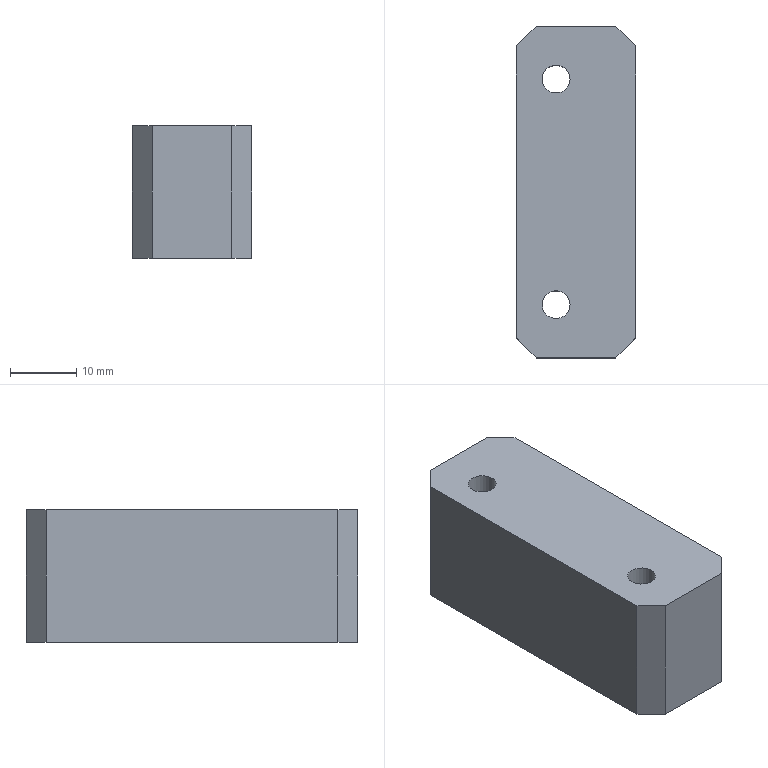Part | NX | 1 solid | 12 faces | box 18 x 50 x 20 mm | volume 17086 mm3 | plane 10 | cylinder 2 | commonest cylinder face diameters 4.2 x2
STEP:
#1=CARTESIAN_POINT('',(-184.109,20.55,354.2));
#2=VERTEX_POINT('',#1);
#3=CARTESIAN_POINT('',(-187.109,17.55,354.2));
#4=VERTEX_POINT('',#3);
#5=CARTESIAN_POINT('',(-184.109,20.55,354.2));
#6=DIRECTION('',(-0.7071,-0.7071,0.));
#7=VECTOR('',#6,1000.);
#8=LINE('',#5,#7);
#9=EDGE_CURVE('',#2,#4,#8,.T.);
#10=ORIENTED_EDGE('',*,*,#9,.T.);
#11=CARTESIAN_POINT('',(-199.109,17.55,354.2));
#12=VERTEX_POINT('',#11);
#13=CARTESIAN_POINT('',(-187.109,17.55,354.2));
#14=DIRECTION('',(-1.,0.,0.));
#15=VECTOR('',#14,1000.);
#16=LINE('',#13,#15);
#17=EDGE_CURVE('',#4,#12,#16,.T.);
#18=ORIENTED_EDGE('',*,*,#17,.T.);
#19=CARTESIAN_POINT('',(-202.109,20.55,354.2));
#20=VERTEX_POINT('',#19);
#21=CARTESIAN_POINT('',(-199.109,17.55,354.2));
#22=DIRECTION('',(-0.7071,0.7071,0.));
#23=VECTOR('',#22,1000.);
#24=LINE('',#21,#23);
#25=EDGE_CURVE('',#12,#20,#24,.T.);
#26=ORIENTED_EDGE('',*,*,#25,.T.);
#27=CARTESIAN_POINT('',(-202.109,64.55,354.2));
#28=VERTEX_POINT('',#27);
#29=CARTESIAN_POINT('',(-202.109,20.55,354.2));
#30=DIRECTION('',(0.,1.,0.));
#31=VECTOR('',#30,1000.);
#32=LINE('',#29,#31);
#33=EDGE_CURVE('',#20,#28,#32,.T.);
#34=ORIENTED_EDGE('',*,*,#33,.T.);
#35=CARTESIAN_POINT('',(-199.109,67.55,354.2));
#36=VERTEX_POINT('',#35);
#37=CARTESIAN_POINT('',(-202.109,64.55,354.2));
#38=DIRECTION('',(0.7071,0.7071,0.));
#39=VECTOR('',#38,1000.);
#40=LINE('',#37,#39);
#41=EDGE_CURVE('',#28,#36,#40,.T.);
#42=ORIENTED_EDGE('',*,*,#41,.T.);
#43=CARTESIAN_POINT('',(-187.109,67.55,354.2));
#44=VERTEX_POINT('',#43);
#45=CARTESIAN_POINT('',(-199.109,67.55,354.2));
#46=DIRECTION('',(1.,0.,0.));
#47=VECTOR('',#46,1000.);
#48=LINE('',#45,#47);
#49=EDGE_CURVE('',#36,#44,#48,.T.);
#50=ORIENTED_EDGE('',*,*,#49,.T.);
#51=CARTESIAN_POINT('',(-184.109,64.55,354.2));
#52=VERTEX_POINT('',#51);
#53=CARTESIAN_POINT('',(-187.109,67.55,354.2));
#54=DIRECTION('',(0.7071,-0.7071,0.));
#55=VECTOR('',#54,1000.);
#56=LINE('',#53,#55);
#57=EDGE_CURVE('',#44,#52,#56,.T.);
#58=ORIENTED_EDGE('',*,*,#57,.T.);
#59=CARTESIAN_POINT('',(-184.109,64.55,354.2));
#60=DIRECTION('',(0.,-1.,0.));
#61=VECTOR('',#60,1000.);
#62=LINE('',#59,#61);
#63=EDGE_CURVE('',#52,#2,#62,.T.);
#64=ORIENTED_EDGE('',*,*,#63,.T.);
#65=EDGE_LOOP('',(#10,#18,#26,#34,#42,#50,#58,#64));
#66=FACE_BOUND('',#65,.T.);
#67=CARTESIAN_POINT('',(-194.009,25.55,354.2));
#68=VERTEX_POINT('',#67);
#69=CARTESIAN_POINT('',(-196.109,25.55,354.2));
#70=DIRECTION('',(0.,0.,1.));
#71=DIRECTION('',(1.,0.,0.));
#72=AXIS2_PLACEMENT_3D('',#69,#70,#71);
#73=CIRCLE('',#72,2.1);
#74=EDGE_CURVE('',#68,#68,#73,.T.);
#75=ORIENTED_EDGE('',*,*,#74,.T.);
#76=EDGE_LOOP('',(#75));
#77=FACE_BOUND('',#76,.T.);
#78=CARTESIAN_POINT('',(-194.009,59.55,354.2));
#79=VERTEX_POINT('',#78);
#80=CARTESIAN_POINT('',(-196.109,59.55,354.2));
#81=DIRECTION('',(0.,0.,1.));
#82=DIRECTION('',(1.,0.,0.));
#83=AXIS2_PLACEMENT_3D('',#80,#81,#82);
#84=CIRCLE('',#83,2.1);
#85=EDGE_CURVE('',#79,#79,#84,.T.);
#86=ORIENTED_EDGE('',*,*,#85,.T.);
#87=EDGE_LOOP('',(#86));
#88=FACE_BOUND('',#87,.T.);
#89=CARTESIAN_POINT('',(1.91,3.142,354.2));
#90=DIRECTION('',(0.,0.,-1.));
#91=DIRECTION('',(0.,-1.,0.));
#92=AXIS2_PLACEMENT_3D('',#89,#90,#91);
#93=PLANE('',#92);
#94=ADVANCED_FACE('',(#66,#77,#88),#93,.T.);
#95=CARTESIAN_POINT('',(-184.109,20.55,374.2));
#96=VERTEX_POINT('',#95);
#97=CARTESIAN_POINT('',(-187.109,17.55,374.2));
#98=VERTEX_POINT('',#97);
#99=CARTESIAN_POINT('',(-184.109,20.55,374.2));
#100=DIRECTION('',(-0.7071,-0.7071,0.));
#101=VECTOR('',#100,1000.);
#102=LINE('',#99,#101);
#103=EDGE_CURVE('',#96,#98,#102,.T.);
#104=ORIENTED_EDGE('',*,*,#103,.F.);
#105=CARTESIAN_POINT('',(-184.109,64.55,374.2));
#106=VERTEX_POINT('',#105);
#107=CARTESIAN_POINT('',(-184.109,64.55,374.2));
#108=DIRECTION('',(0.,-1.,0.));
#109=VECTOR('',#108,1000.);
#110=LINE('',#107,#109);
#111=EDGE_CURVE('',#106,#96,#110,.T.);
#112=ORIENTED_EDGE('',*,*,#111,.F.);
#113=CARTESIAN_POINT('',(-187.109,67.55,374.2));
#114=VERTEX_POINT('',#113);
#115=CARTESIAN_POINT('',(-187.109,67.55,374.2));
#116=DIRECTION('',(0.7071,-0.7071,0.));
#117=VECTOR('',#116,1000.);
#118=LINE('',#115,#117);
#119=EDGE_CURVE('',#114,#106,#118,.T.);
#120=ORIENTED_EDGE('',*,*,#119,.F.);
#121=CARTESIAN_POINT('',(-199.109,67.55,374.2));
#122=VERTEX_POINT('',#121);
#123=CARTESIAN_POINT('',(-199.109,67.55,374.2));
#124=DIRECTION('',(1.,0.,0.));
#125=VECTOR('',#124,1000.);
#126=LINE('',#123,#125);
#127=EDGE_CURVE('',#122,#114,#126,.T.);
#128=ORIENTED_EDGE('',*,*,#127,.F.);
#129=CARTESIAN_POINT('',(-202.109,64.55,374.2));
#130=VERTEX_POINT('',#129);
#131=CARTESIAN_POINT('',(-202.109,64.55,374.2));
#132=DIRECTION('',(0.7071,0.7071,0.));
#133=VECTOR('',#132,1000.);
#134=LINE('',#131,#133);
#135=EDGE_CURVE('',#130,#122,#134,.T.);
#136=ORIENTED_EDGE('',*,*,#135,.F.);
#137=CARTESIAN_POINT('',(-202.109,20.55,374.2));
#138=VERTEX_POINT('',#137);
#139=CARTESIAN_POINT('',(-202.109,20.55,374.2));
#140=DIRECTION('',(0.,1.,0.));
#141=VECTOR('',#140,1000.);
#142=LINE('',#139,#141);
#143=EDGE_CURVE('',#138,#130,#142,.T.);
#144=ORIENTED_EDGE('',*,*,#143,.F.);
#145=CARTESIAN_POINT('',(-199.109,17.55,374.2));
#146=VERTEX_POINT('',#145);
#147=CARTESIAN_POINT('',(-199.109,17.55,374.2));
#148=DIRECTION('',(-0.7071,0.7071,0.));
#149=VECTOR('',#148,1000.);
#150=LINE('',#147,#149);
#151=EDGE_CURVE('',#146,#138,#150,.T.);
#152=ORIENTED_EDGE('',*,*,#151,.F.);
#153=CARTESIAN_POINT('',(-187.109,17.55,374.2));
#154=DIRECTION('',(-1.,0.,0.));
#155=VECTOR('',#154,1000.);
#156=LINE('',#153,#155);
#157=EDGE_CURVE('',#98,#146,#156,.T.);
#158=ORIENTED_EDGE('',*,*,#157,.F.);
#159=EDGE_LOOP('',(#104,#112,#120,#128,#136,#144,#152,#158));
#160=FACE_BOUND('',#159,.T.);
#161=CARTESIAN_POINT('',(-194.009,25.55,374.2));
#162=VERTEX_POINT('',#161);
#163=CARTESIAN_POINT('',(-196.109,25.55,374.2));
#164=DIRECTION('',(0.,0.,1.));
#165=DIRECTION('',(1.,0.,0.));
#166=AXIS2_PLACEMENT_3D('',#163,#164,#165);
#167=CIRCLE('',#166,2.1);
#168=EDGE_CURVE('',#162,#162,#167,.T.);
#169=ORIENTED_EDGE('',*,*,#168,.F.);
#170=EDGE_LOOP('',(#169));
#171=FACE_BOUND('',#170,.T.);
#172=CARTESIAN_POINT('',(-194.009,59.55,374.2));
#173=VERTEX_POINT('',#172);
#174=CARTESIAN_POINT('',(-196.109,59.55,374.2));
#175=DIRECTION('',(0.,0.,1.));
#176=DIRECTION('',(1.,0.,0.));
#177=AXIS2_PLACEMENT_3D('',#174,#175,#176);
#178=CIRCLE('',#177,2.1);
#179=EDGE_CURVE('',#173,#173,#178,.T.);
#180=ORIENTED_EDGE('',*,*,#179,.F.);
#181=EDGE_LOOP('',(#180));
#182=FACE_BOUND('',#181,.T.);
#183=CARTESIAN_POINT('',(1.91,3.142,374.2));
#184=DIRECTION('',(0.,0.,-1.));
#185=DIRECTION('',(0.,-1.,0.));
#186=AXIS2_PLACEMENT_3D('',#183,#184,#185);
#187=PLANE('',#186);
#188=ADVANCED_FACE('',(#160,#171,#182),#187,.F.);
#189=ORIENTED_EDGE('',*,*,#17,.F.);
#190=CARTESIAN_POINT('',(-187.109,17.55,374.2));
#191=DIRECTION('',(0.,0.,-1.));
#192=VECTOR('',#191,1000.);
#193=LINE('',#190,#192);
#194=EDGE_CURVE('',#98,#4,#193,.T.);
#195=ORIENTED_EDGE('',*,*,#194,.F.);
#196=ORIENTED_EDGE('',*,*,#157,.T.);
#197=CARTESIAN_POINT('',(-199.109,17.55,374.2));
#198=DIRECTION('',(0.,0.,-1.));
#199=VECTOR('',#198,1000.);
#200=LINE('',#197,#199);
#201=EDGE_CURVE('',#146,#12,#200,.T.);
#202=ORIENTED_EDGE('',*,*,#201,.T.);
#203=EDGE_LOOP('',(#189,#195,#196,#202));
#204=FACE_BOUND('',#203,.T.);
#205=CARTESIAN_POINT('',(-187.109,17.55,374.2));
#206=DIRECTION('',(0.,-1.,0.));
#207=DIRECTION('',(0.,0.,-1.));
#208=AXIS2_PLACEMENT_3D('',#205,#206,#207);
#209=PLANE('',#208);
#210=ADVANCED_FACE('',(#204),#209,.T.);
#211=ORIENTED_EDGE('',*,*,#25,.F.);
#212=ORIENTED_EDGE('',*,*,#201,.F.);
#213=ORIENTED_EDGE('',*,*,#151,.T.);
#214=CARTESIAN_POINT('',(-202.109,20.55,374.2));
#215=DIRECTION('',(0.,0.,-1.));
#216=VECTOR('',#215,1000.);
#217=LINE('',#214,#216);
#218=EDGE_CURVE('',#138,#20,#217,.T.);
#219=ORIENTED_EDGE('',*,*,#218,.T.);
#220=EDGE_LOOP('',(#211,#212,#213,#219));
#221=FACE_BOUND('',#220,.T.);
#222=CARTESIAN_POINT('',(-199.109,17.55,374.2));
#223=DIRECTION('',(-0.7071,-0.7071,0.));
#224=DIRECTION('',(-0.7071,0.7071,0.));
#225=AXIS2_PLACEMENT_3D('',#222,#223,#224);
#226=PLANE('',#225);
#227=ADVANCED_FACE('',(#221),#226,.T.);
#228=ORIENTED_EDGE('',*,*,#33,.F.);
#229=ORIENTED_EDGE('',*,*,#218,.F.);
#230=ORIENTED_EDGE('',*,*,#143,.T.);
#231=CARTESIAN_POINT('',(-202.109,64.55,374.2));
#232=DIRECTION('',(0.,0.,-1.));
#233=VECTOR('',#232,1000.);
#234=LINE('',#231,#233);
#235=EDGE_CURVE('',#130,#28,#234,.T.);
#236=ORIENTED_EDGE('',*,*,#235,.T.);
#237=EDGE_LOOP('',(#228,#229,#230,#236));
#238=FACE_BOUND('',#237,.T.);
#239=CARTESIAN_POINT('',(-202.109,20.55,374.2));
#240=DIRECTION('',(-1.,0.,0.));
#241=DIRECTION('',(0.,0.,1.));
#242=AXIS2_PLACEMENT_3D('',#239,#240,#241);
#243=PLANE('',#242);
#244=ADVANCED_FACE('',(#238),#243,.T.);
#245=ORIENTED_EDGE('',*,*,#41,.F.);
#246=ORIENTED_EDGE('',*,*,#235,.F.);
#247=ORIENTED_EDGE('',*,*,#135,.T.);
#248=CARTESIAN_POINT('',(-199.109,67.55,374.2));
#249=DIRECTION('',(0.,0.,-1.));
#250=VECTOR('',#249,1000.);
#251=LINE('',#248,#250);
#252=EDGE_CURVE('',#122,#36,#251,.T.);
#253=ORIENTED_EDGE('',*,*,#252,.T.);
#254=EDGE_LOOP('',(#245,#246,#247,#253));
#255=FACE_BOUND('',#254,.T.);
#256=CARTESIAN_POINT('',(-202.109,64.55,374.2));
#257=DIRECTION('',(-0.7071,0.7071,0.));
#258=DIRECTION('',(0.,0.,1.));
#259=AXIS2_PLACEMENT_3D('',#256,#257,#258);
#260=PLANE('',#259);
#261=ADVANCED_FACE('',(#255),#260,.T.);
#262=ORIENTED_EDGE('',*,*,#49,.F.);
#263=ORIENTED_EDGE('',*,*,#252,.F.);
#264=ORIENTED_EDGE('',*,*,#127,.T.);
#265=CARTESIAN_POINT('',(-187.109,67.55,374.2));
#266=DIRECTION('',(0.,0.,-1.));
#267=VECTOR('',#266,1000.);
#268=LINE('',#265,#267);
#269=EDGE_CURVE('',#114,#44,#268,.T.);
#270=ORIENTED_EDGE('',*,*,#269,.T.);
#271=EDGE_LOOP('',(#262,#263,#264,#270));
#272=FACE_BOUND('',#271,.T.);
#273=CARTESIAN_POINT('',(-199.109,67.55,374.2));
#274=DIRECTION('',(0.,1.,0.));
#275=DIRECTION('',(1.,0.,0.));
#276=AXIS2_PLACEMENT_3D('',#273,#274,#275);
#277=PLANE('',#276);
#278=ADVANCED_FACE('',(#272),#277,.T.);
#279=ORIENTED_EDGE('',*,*,#57,.F.);
#280=ORIENTED_EDGE('',*,*,#269,.F.);
#281=ORIENTED_EDGE('',*,*,#119,.T.);
#282=CARTESIAN_POINT('',(-184.109,64.55,374.2));
#283=DIRECTION('',(0.,0.,-1.));
#284=VECTOR('',#283,1000.);
#285=LINE('',#282,#284);
#286=EDGE_CURVE('',#106,#52,#285,.T.);
#287=ORIENTED_EDGE('',*,*,#286,.T.);
#288=EDGE_LOOP('',(#279,#280,#281,#287));
#289=FACE_BOUND('',#288,.T.);
#290=CARTESIAN_POINT('',(-187.109,67.55,374.2));
#291=DIRECTION('',(0.7071,0.7071,0.));
#292=DIRECTION('',(0.,0.,-1.));
#293=AXIS2_PLACEMENT_3D('',#290,#291,#292);
#294=PLANE('',#293);
#295=ADVANCED_FACE('',(#289),#294,.T.);
#296=ORIENTED_EDGE('',*,*,#63,.F.);
#297=ORIENTED_EDGE('',*,*,#286,.F.);
#298=ORIENTED_EDGE('',*,*,#111,.T.);
#299=CARTESIAN_POINT('',(-184.109,20.55,374.2));
#300=DIRECTION('',(0.,0.,-1.));
#301=VECTOR('',#300,1000.);
#302=LINE('',#299,#301);
#303=EDGE_CURVE('',#96,#2,#302,.T.);
#304=ORIENTED_EDGE('',*,*,#303,.T.);
#305=EDGE_LOOP('',(#296,#297,#298,#304));
#306=FACE_BOUND('',#305,.T.);
#307=CARTESIAN_POINT('',(-184.109,64.55,374.2));
#308=DIRECTION('',(1.,0.,0.));
#309=DIRECTION('',(0.,1.,0.));
#310=AXIS2_PLACEMENT_3D('',#307,#308,#309);
#311=PLANE('',#310);
#312=ADVANCED_FACE('',(#306),#311,.T.);
#313=ORIENTED_EDGE('',*,*,#9,.F.);
#314=ORIENTED_EDGE('',*,*,#303,.F.);
#315=ORIENTED_EDGE('',*,*,#103,.T.);
#316=ORIENTED_EDGE('',*,*,#194,.T.);
#317=EDGE_LOOP('',(#313,#314,#315,#316));
#318=FACE_BOUND('',#317,.T.);
#319=CARTESIAN_POINT('',(-184.109,20.55,374.2));
#320=DIRECTION('',(0.7071,-0.7071,0.));
#321=DIRECTION('',(0.,0.,-1.));
#322=AXIS2_PLACEMENT_3D('',#319,#320,#321);
#323=PLANE('',#322);
#324=ADVANCED_FACE('',(#318),#323,.T.);
#325=ORIENTED_EDGE('',*,*,#74,.F.);
#326=EDGE_LOOP('',(#325));
#327=FACE_BOUND('',#326,.T.);
#328=ORIENTED_EDGE('',*,*,#168,.T.);
#329=EDGE_LOOP('',(#328));
#330=FACE_BOUND('',#329,.T.);
#331=CARTESIAN_POINT('',(-196.109,25.55,374.2));
#332=DIRECTION('',(0.,0.,1.));
#333=DIRECTION('',(1.,0.,0.));
#334=AXIS2_PLACEMENT_3D('',#331,#332,#333);
#335=CYLINDRICAL_SURFACE('',#334,2.1);
#336=ADVANCED_FACE('',(#327,#330),#335,.F.);
#337=ORIENTED_EDGE('',*,*,#85,.F.);
#338=EDGE_LOOP('',(#337));
#339=FACE_BOUND('',#338,.T.);
#340=ORIENTED_EDGE('',*,*,#179,.T.);
#341=EDGE_LOOP('',(#340));
#342=FACE_BOUND('',#341,.T.);
#343=CARTESIAN_POINT('',(-196.109,59.55,374.2));
#344=DIRECTION('',(0.,0.,1.));
#345=DIRECTION('',(1.,0.,0.));
#346=AXIS2_PLACEMENT_3D('',#343,#344,#345);
#347=CYLINDRICAL_SURFACE('',#346,2.1);
#348=ADVANCED_FACE('',(#339,#342),#347,.F.);
#349=CLOSED_SHELL('',(#94,#188,#210,#227,#244,#261,#278,#295,#312,#324,#336,#348));
#350=MANIFOLD_SOLID_BREP('',#349);
#351=(LENGTH_UNIT()NAMED_UNIT(*)SI_UNIT(.MILLI.,.METRE.));
#352=UNCERTAINTY_MEASURE_WITH_UNIT(LENGTH_MEASURE(0.00001),#351,'','');
#353=(NAMED_UNIT(*)PLANE_ANGLE_UNIT()SI_UNIT($,.RADIAN.));
#354=(NAMED_UNIT(*)SI_UNIT($,.STERADIAN.)SOLID_ANGLE_UNIT());
#355=(GEOMETRIC_REPRESENTATION_CONTEXT(3)GLOBAL_UNCERTAINTY_ASSIGNED_CONTEXT((#352))GLOBAL_UNIT_ASSIGNED_CONTEXT((#351,#353,#354))REPRESENTATION_CONTEXT('',''));
#356=ADVANCED_BREP_SHAPE_REPRESENTATION('',(#350),#355);